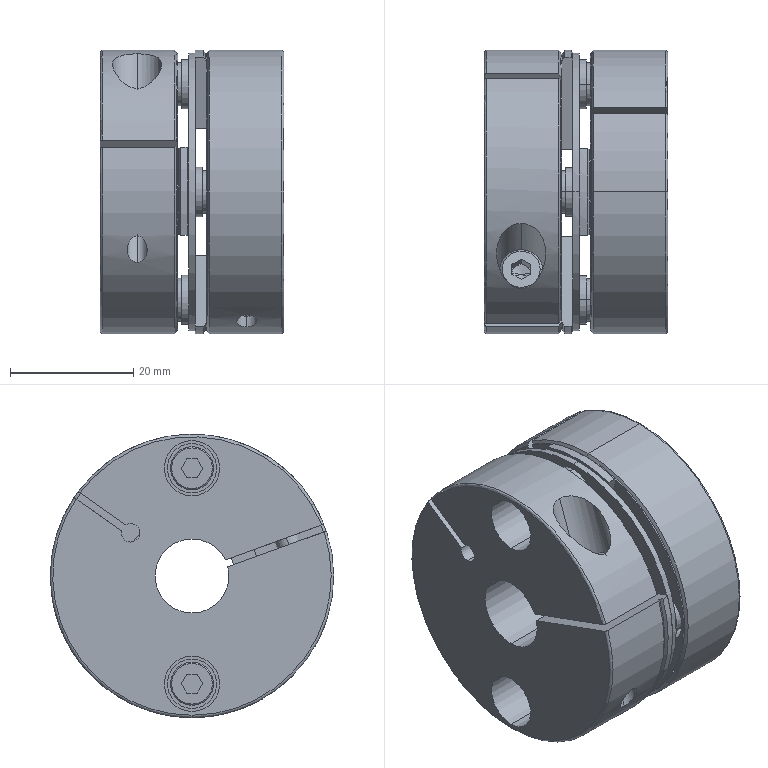Part | STEP file | 001-003-C-SCPS46-12-14 | 3 solids | 230 faces | box 29.8 x 46 x 46 mm | volume 36563 mm3 | plane 98 | cylinder 74 | cone 38 | torus 20 | commonest cylinder face diameters 7 x12 8 x12 46 x12 3.242 x8 9 x8 3 x6